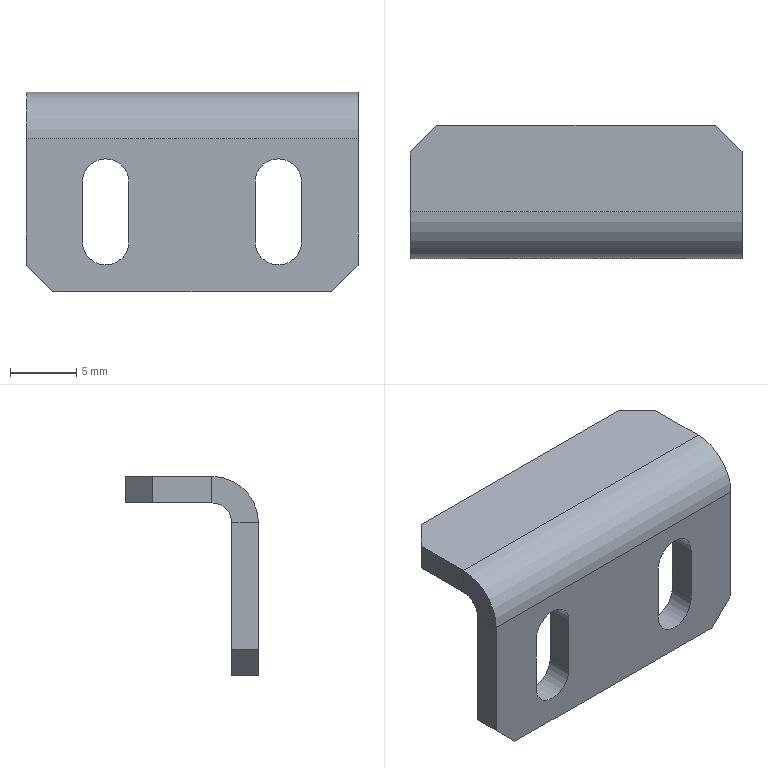Part | STEP file | 227H056378 BKT_Default | 1 solid | 28 faces | box 25 x 10 x 15 mm | volume 978.865 mm3 | plane 20 | cylinder 8 | commonest cylinder face diameters 3.5 x6 3 x1 7 x1